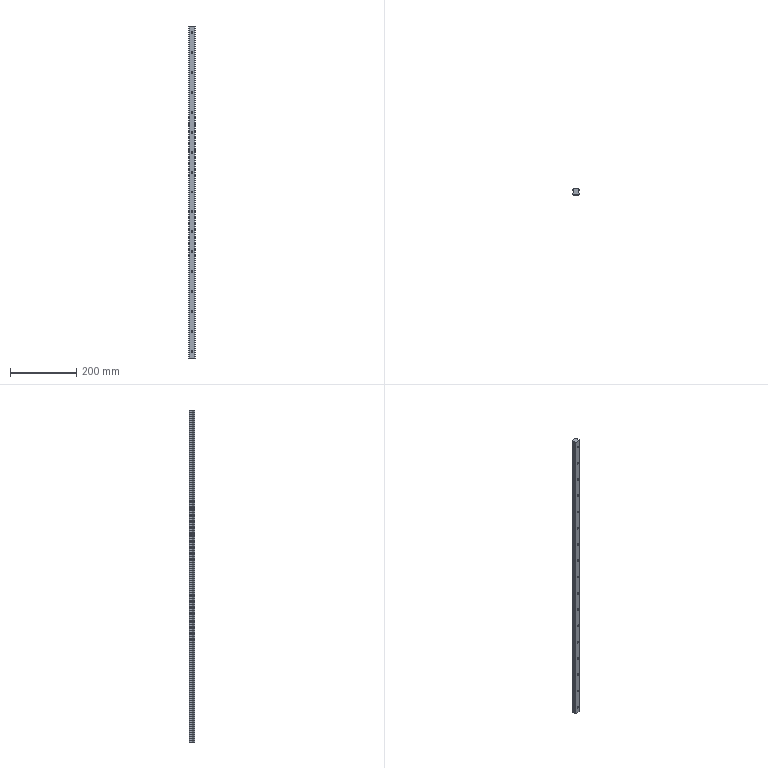Part | SolidWorks | features BaseBody 1 | 1 solid | 129 faces | box 20 x 17.5 x 1000 mm | volume 284337 mm3 | cylinder 90 | plane 39 | commonest cylinder face diameters 6 x34 9.5 x34 1 x12 2 x6 4.06 x4